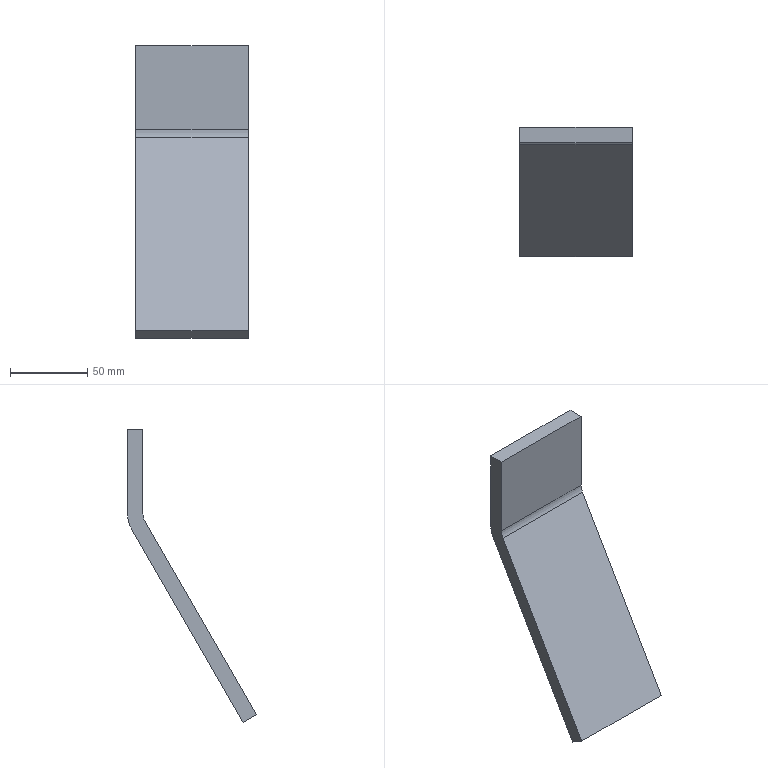Part | STEP file | VD-SYL0380DJ1006_1_5-5_VD-SYL03 | 1 solid | 10 faces | box 73 x 83.716 x 190 mm | volume 151290 mm3 | plane 8 | cylinder 2 | commonest cylinder face diameters 20 x1 40 x1
STEP:
#1=CARTESIAN_POINT('',(36.5,-2.679,-64.641));
#2=VERTEX_POINT('',#1);
#3=CARTESIAN_POINT('',(-36.5,-2.679,-64.641));
#4=VERTEX_POINT('',#3);
#5=CARTESIAN_POINT('',(36.5,-2.679,-64.641));
#6=DIRECTION('',(-1.,0.,0.));
#7=VECTOR('',#6,1000.);
#8=LINE('',#5,#7);
#9=EDGE_CURVE('',#2,#4,#8,.T.);
#10=ORIENTED_EDGE('',*,*,#9,.T.);
#11=CARTESIAN_POINT('',(-36.5,0.,-54.641));
#12=VERTEX_POINT('',#11);
#13=CARTESIAN_POINT('',(-36.5,-20.,-54.641));
#14=DIRECTION('',(-1.,0.,0.));
#15=DIRECTION('',(0.,1.,0.));
#16=AXIS2_PLACEMENT_3D('',#13,#14,#15);
#17=CIRCLE('',#16,20.);
#18=EDGE_CURVE('',#12,#4,#17,.T.);
#19=ORIENTED_EDGE('',*,*,#18,.F.);
#20=CARTESIAN_POINT('',(36.5,0.,-54.641));
#21=VERTEX_POINT('',#20);
#22=CARTESIAN_POINT('',(-36.5,0.,-54.641));
#23=DIRECTION('',(1.,0.,0.));
#24=VECTOR('',#23,1000.);
#25=LINE('',#22,#24);
#26=EDGE_CURVE('',#12,#21,#25,.T.);
#27=ORIENTED_EDGE('',*,*,#26,.T.);
#28=CARTESIAN_POINT('',(36.5,-20.,-54.641));
#29=DIRECTION('',(1.,0.,0.));
#30=DIRECTION('',(0.,0.866,-0.5));
#31=AXIS2_PLACEMENT_3D('',#28,#29,#30);
#32=CIRCLE('',#31,20.);
#33=EDGE_CURVE('',#2,#21,#32,.T.);
#34=ORIENTED_EDGE('',*,*,#33,.F.);
#35=EDGE_LOOP('',(#10,#19,#27,#34));
#36=FACE_OUTER_BOUND('',#35,.T.);
#37=CARTESIAN_POINT('',(212.726,-20.,-54.641));
#38=DIRECTION('',(-1.,0.,0.));
#39=DIRECTION('',(0.,0.,1.));
#40=AXIS2_PLACEMENT_3D('',#37,#38,#39);
#41=CYLINDRICAL_SURFACE('',#40,20.);
#42=ADVANCED_FACE('',(#36),#41,.T.);
#43=ORIENTED_EDGE('',*,*,#26,.F.);
#44=CARTESIAN_POINT('',(-36.5,0.,0.));
#45=VERTEX_POINT('',#44);
#46=CARTESIAN_POINT('',(-36.5,0.,-54.641));
#47=DIRECTION('',(0.,0.,1.));
#48=VECTOR('',#47,1000.);
#49=LINE('',#46,#48);
#50=EDGE_CURVE('',#12,#45,#49,.T.);
#51=ORIENTED_EDGE('',*,*,#50,.T.);
#52=CARTESIAN_POINT('',(36.5,0.,0.));
#53=VERTEX_POINT('',#52);
#54=CARTESIAN_POINT('',(-36.5,0.,0.));
#55=DIRECTION('',(1.,0.,0.));
#56=VECTOR('',#55,1000.);
#57=LINE('',#54,#56);
#58=EDGE_CURVE('',#45,#53,#57,.T.);
#59=ORIENTED_EDGE('',*,*,#58,.T.);
#60=CARTESIAN_POINT('',(36.5,0.,-54.641));
#61=DIRECTION('',(0.,0.,1.));
#62=VECTOR('',#61,1000.);
#63=LINE('',#60,#62);
#64=EDGE_CURVE('',#21,#53,#63,.T.);
#65=ORIENTED_EDGE('',*,*,#64,.F.);
#66=EDGE_LOOP('',(#43,#51,#59,#65));
#67=FACE_OUTER_BOUND('',#66,.T.);
#68=CARTESIAN_POINT('',(-36.5,0.,-60.));
#69=DIRECTION('',(0.,1.,0.));
#70=DIRECTION('',(1.,0.,0.));
#71=AXIS2_PLACEMENT_3D('',#68,#69,#70);
#72=PLANE('',#71);
#73=ADVANCED_FACE('',(#67),#72,.T.);
#74=ORIENTED_EDGE('',*,*,#58,.F.);
#75=CARTESIAN_POINT('',(-36.5,-10.,0.));
#76=VERTEX_POINT('',#75);
#77=CARTESIAN_POINT('',(-36.5,0.,0.));
#78=DIRECTION('',(0.,-1.,0.));
#79=VECTOR('',#78,1000.);
#80=LINE('',#77,#79);
#81=EDGE_CURVE('',#45,#76,#80,.T.);
#82=ORIENTED_EDGE('',*,*,#81,.T.);
#83=CARTESIAN_POINT('',(36.5,-10.,0.));
#84=VERTEX_POINT('',#83);
#85=CARTESIAN_POINT('',(36.5,-10.,0.));
#86=DIRECTION('',(-1.,0.,0.));
#87=VECTOR('',#86,1000.);
#88=LINE('',#85,#87);
#89=EDGE_CURVE('',#84,#76,#88,.T.);
#90=ORIENTED_EDGE('',*,*,#89,.F.);
#91=CARTESIAN_POINT('',(36.5,0.,0.));
#92=DIRECTION('',(0.,-1.,0.));
#93=VECTOR('',#92,1000.);
#94=LINE('',#91,#93);
#95=EDGE_CURVE('',#53,#84,#94,.T.);
#96=ORIENTED_EDGE('',*,*,#95,.F.);
#97=EDGE_LOOP('',(#74,#82,#90,#96));
#98=FACE_OUTER_BOUND('',#97,.T.);
#99=CARTESIAN_POINT('',(0.,-5.,0.));
#100=DIRECTION('',(0.,0.,1.));
#101=DIRECTION('',(1.,0.,0.));
#102=AXIS2_PLACEMENT_3D('',#99,#100,#101);
#103=PLANE('',#102);
#104=ADVANCED_FACE('',(#98),#103,.T.);
#105=CARTESIAN_POINT('',(-36.5,-10.,-54.641));
#106=VERTEX_POINT('',#105);
#107=CARTESIAN_POINT('',(-36.5,-10.,0.));
#108=DIRECTION('',(0.,0.,-1.));
#109=VECTOR('',#108,1000.);
#110=LINE('',#107,#109);
#111=EDGE_CURVE('',#76,#106,#110,.T.);
#112=ORIENTED_EDGE('',*,*,#111,.T.);
#113=CARTESIAN_POINT('',(36.5,-10.,-54.641));
#114=VERTEX_POINT('',#113);
#115=CARTESIAN_POINT('',(36.5,-10.,-54.641));
#116=DIRECTION('',(-1.,0.,0.));
#117=VECTOR('',#116,1000.);
#118=LINE('',#115,#117);
#119=EDGE_CURVE('',#114,#106,#118,.T.);
#120=ORIENTED_EDGE('',*,*,#119,.F.);
#121=CARTESIAN_POINT('',(36.5,-10.,-54.641));
#122=DIRECTION('',(0.,0.,1.));
#123=VECTOR('',#122,1000.);
#124=LINE('',#121,#123);
#125=EDGE_CURVE('',#114,#84,#124,.T.);
#126=ORIENTED_EDGE('',*,*,#125,.T.);
#127=ORIENTED_EDGE('',*,*,#89,.T.);
#128=EDGE_LOOP('',(#112,#120,#126,#127));
#129=FACE_OUTER_BOUND('',#128,.T.);
#130=CARTESIAN_POINT('',(-36.5,-10.,-60.));
#131=DIRECTION('',(0.,1.,0.));
#132=DIRECTION('',(1.,0.,0.));
#133=AXIS2_PLACEMENT_3D('',#130,#131,#132);
#134=PLANE('',#133);
#135=ADVANCED_FACE('',(#129),#134,.F.);
#136=CARTESIAN_POINT('',(-36.5,-11.34,-59.641));
#137=VERTEX_POINT('',#136);
#138=CARTESIAN_POINT('',(-36.5,-20.,-54.641));
#139=DIRECTION('',(1.,0.,0.));
#140=DIRECTION('',(0.,0.866,-0.5));
#141=AXIS2_PLACEMENT_3D('',#138,#139,#140);
#142=CIRCLE('',#141,10.);
#143=EDGE_CURVE('',#137,#106,#142,.T.);
#144=ORIENTED_EDGE('',*,*,#143,.F.);
#145=CARTESIAN_POINT('',(36.5,-11.34,-59.641));
#146=VERTEX_POINT('',#145);
#147=CARTESIAN_POINT('',(-36.5,-11.34,-59.641));
#148=DIRECTION('',(1.,0.,0.));
#149=VECTOR('',#148,1000.);
#150=LINE('',#147,#149);
#151=EDGE_CURVE('',#137,#146,#150,.T.);
#152=ORIENTED_EDGE('',*,*,#151,.T.);
#153=CARTESIAN_POINT('',(36.5,-20.,-54.641));
#154=DIRECTION('',(-1.,0.,0.));
#155=DIRECTION('',(0.,1.,0.));
#156=AXIS2_PLACEMENT_3D('',#153,#154,#155);
#157=CIRCLE('',#156,10.);
#158=EDGE_CURVE('',#114,#146,#157,.T.);
#159=ORIENTED_EDGE('',*,*,#158,.F.);
#160=ORIENTED_EDGE('',*,*,#119,.T.);
#161=EDGE_LOOP('',(#144,#152,#159,#160));
#162=FACE_OUTER_BOUND('',#161,.T.);
#163=CARTESIAN_POINT('',(212.726,-20.,-54.641));
#164=DIRECTION('',(-1.,0.,0.));
#165=DIRECTION('',(0.,0.,1.));
#166=AXIS2_PLACEMENT_3D('',#163,#164,#165);
#167=CYLINDRICAL_SURFACE('',#166,10.);
#168=ADVANCED_FACE('',(#162),#167,.F.);
#169=CARTESIAN_POINT('',(36.5,-75.056,-190.));
#170=VERTEX_POINT('',#169);
#171=CARTESIAN_POINT('',(36.5,-75.056,-190.));
#172=DIRECTION('',(0.,0.5,0.866));
#173=VECTOR('',#172,1000.);
#174=LINE('',#171,#173);
#175=EDGE_CURVE('',#170,#2,#174,.T.);
#176=ORIENTED_EDGE('',*,*,#175,.T.);
#177=ORIENTED_EDGE('',*,*,#33,.T.);
#178=ORIENTED_EDGE('',*,*,#64,.T.);
#179=ORIENTED_EDGE('',*,*,#95,.T.);
#180=ORIENTED_EDGE('',*,*,#125,.F.);
#181=ORIENTED_EDGE('',*,*,#158,.T.);
#182=CARTESIAN_POINT('',(36.5,-83.716,-185.));
#183=VERTEX_POINT('',#182);
#184=CARTESIAN_POINT('',(36.5,-11.34,-59.641));
#185=DIRECTION('',(0.,-0.5,-0.866));
#186=VECTOR('',#185,1000.);
#187=LINE('',#184,#186);
#188=EDGE_CURVE('',#146,#183,#187,.T.);
#189=ORIENTED_EDGE('',*,*,#188,.T.);
#190=CARTESIAN_POINT('',(36.5,-83.716,-185.));
#191=DIRECTION('',(0.,0.866,-0.5));
#192=VECTOR('',#191,1000.);
#193=LINE('',#190,#192);
#194=EDGE_CURVE('',#183,#170,#193,.T.);
#195=ORIENTED_EDGE('',*,*,#194,.T.);
#196=EDGE_LOOP('',(#176,#177,#178,#179,#180,#181,#189,#195));
#197=FACE_OUTER_BOUND('',#196,.T.);
#198=CARTESIAN_POINT('',(36.5,-42.193,-123.08));
#199=DIRECTION('',(-1.,0.,0.));
#200=DIRECTION('',(0.,0.,1.));
#201=AXIS2_PLACEMENT_3D('',#198,#199,#200);
#202=PLANE('',#201);
#203=ADVANCED_FACE('',(#197),#202,.F.);
#204=ORIENTED_EDGE('',*,*,#9,.F.);
#205=ORIENTED_EDGE('',*,*,#175,.F.);
#206=CARTESIAN_POINT('',(-36.5,-75.056,-190.));
#207=VERTEX_POINT('',#206);
#208=CARTESIAN_POINT('',(-36.5,-75.056,-190.));
#209=DIRECTION('',(1.,0.,0.));
#210=VECTOR('',#209,1000.);
#211=LINE('',#208,#210);
#212=EDGE_CURVE('',#207,#170,#211,.T.);
#213=ORIENTED_EDGE('',*,*,#212,.F.);
#214=CARTESIAN_POINT('',(-36.5,-2.679,-64.641));
#215=DIRECTION('',(0.,-0.5,-0.866));
#216=VECTOR('',#215,1000.);
#217=LINE('',#214,#216);
#218=EDGE_CURVE('',#4,#207,#217,.T.);
#219=ORIENTED_EDGE('',*,*,#218,.F.);
#220=EDGE_LOOP('',(#204,#205,#213,#219));
#221=FACE_OUTER_BOUND('',#220,.T.);
#222=CARTESIAN_POINT('',(-36.5,-75.056,-190.));
#223=DIRECTION('',(0.,0.866,-0.5));
#224=DIRECTION('',(-1.,0.,0.));
#225=AXIS2_PLACEMENT_3D('',#222,#223,#224);
#226=PLANE('',#225);
#227=ADVANCED_FACE('',(#221),#226,.T.);
#228=ORIENTED_EDGE('',*,*,#143,.T.);
#229=ORIENTED_EDGE('',*,*,#111,.F.);
#230=ORIENTED_EDGE('',*,*,#81,.F.);
#231=ORIENTED_EDGE('',*,*,#50,.F.);
#232=ORIENTED_EDGE('',*,*,#18,.T.);
#233=ORIENTED_EDGE('',*,*,#218,.T.);
#234=CARTESIAN_POINT('',(-36.5,-83.716,-185.));
#235=VERTEX_POINT('',#234);
#236=CARTESIAN_POINT('',(-36.5,-75.056,-190.));
#237=DIRECTION('',(0.,-0.866,0.5));
#238=VECTOR('',#237,1000.);
#239=LINE('',#236,#238);
#240=EDGE_CURVE('',#207,#235,#239,.T.);
#241=ORIENTED_EDGE('',*,*,#240,.T.);
#242=CARTESIAN_POINT('',(-36.5,-83.716,-185.));
#243=DIRECTION('',(0.,0.5,0.866));
#244=VECTOR('',#243,1000.);
#245=LINE('',#242,#244);
#246=EDGE_CURVE('',#235,#137,#245,.T.);
#247=ORIENTED_EDGE('',*,*,#246,.T.);
#248=EDGE_LOOP('',(#228,#229,#230,#231,#232,#233,#241,#247));
#249=FACE_OUTER_BOUND('',#248,.T.);
#250=CARTESIAN_POINT('',(-36.5,-42.193,-123.08));
#251=DIRECTION('',(-1.,0.,0.));
#252=DIRECTION('',(0.,0.,1.));
#253=AXIS2_PLACEMENT_3D('',#250,#251,#252);
#254=PLANE('',#253);
#255=ADVANCED_FACE('',(#249),#254,.T.);
#256=ORIENTED_EDGE('',*,*,#188,.F.);
#257=ORIENTED_EDGE('',*,*,#151,.F.);
#258=ORIENTED_EDGE('',*,*,#246,.F.);
#259=CARTESIAN_POINT('',(-36.5,-83.716,-185.));
#260=DIRECTION('',(1.,0.,0.));
#261=VECTOR('',#260,1000.);
#262=LINE('',#259,#261);
#263=EDGE_CURVE('',#235,#183,#262,.T.);
#264=ORIENTED_EDGE('',*,*,#263,.T.);
#265=EDGE_LOOP('',(#256,#257,#258,#264));
#266=FACE_OUTER_BOUND('',#265,.T.);
#267=CARTESIAN_POINT('',(-36.5,-83.716,-185.));
#268=DIRECTION('',(0.,0.866,-0.5));
#269=DIRECTION('',(-1.,0.,0.));
#270=AXIS2_PLACEMENT_3D('',#267,#268,#269);
#271=PLANE('',#270);
#272=ADVANCED_FACE('',(#266),#271,.F.);
#273=ORIENTED_EDGE('',*,*,#240,.F.);
#274=ORIENTED_EDGE('',*,*,#212,.T.);
#275=ORIENTED_EDGE('',*,*,#194,.F.);
#276=ORIENTED_EDGE('',*,*,#263,.F.);
#277=EDGE_LOOP('',(#273,#274,#275,#276));
#278=FACE_OUTER_BOUND('',#277,.T.);
#279=CARTESIAN_POINT('',(0.,-79.386,-187.5));
#280=DIRECTION('',(0.,0.5,0.866));
#281=DIRECTION('',(1.,0.,0.));
#282=AXIS2_PLACEMENT_3D('',#279,#280,#281);
#283=PLANE('',#282);
#284=ADVANCED_FACE('',(#278),#283,.F.);
#285=CLOSED_SHELL('',(#42,#73,#104,#135,#168,#203,#227,#255,#272,#284));
#286=MANIFOLD_SOLID_BREP('',#285);
#287=CARTESIAN_POINT('',(0.,0.,0.));
#288=DIRECTION('',(0.,0.,1.));
#289=DIRECTION('',(1.,0.,0.));
#290=AXIS2_PLACEMENT_3D('',#287,#288,#289);
#291=(LENGTH_UNIT()NAMED_UNIT(*)SI_UNIT(.MILLI.,.METRE.));
#292=UNCERTAINTY_MEASURE_WITH_UNIT(LENGTH_MEASURE(0.00001),#291,'','');
#293=(NAMED_UNIT(*)PLANE_ANGLE_UNIT()SI_UNIT($,.RADIAN.));
#294=(NAMED_UNIT(*)SI_UNIT($,.STERADIAN.)SOLID_ANGLE_UNIT());
#295=(GEOMETRIC_REPRESENTATION_CONTEXT(3)GLOBAL_UNCERTAINTY_ASSIGNED_CONTEXT((#292))GLOBAL_UNIT_ASSIGNED_CONTEXT((#291,#293,#294))REPRESENTATION_CONTEXT('',''));
#296=ADVANCED_BREP_SHAPE_REPRESENTATION('',(#286,#290),#295);